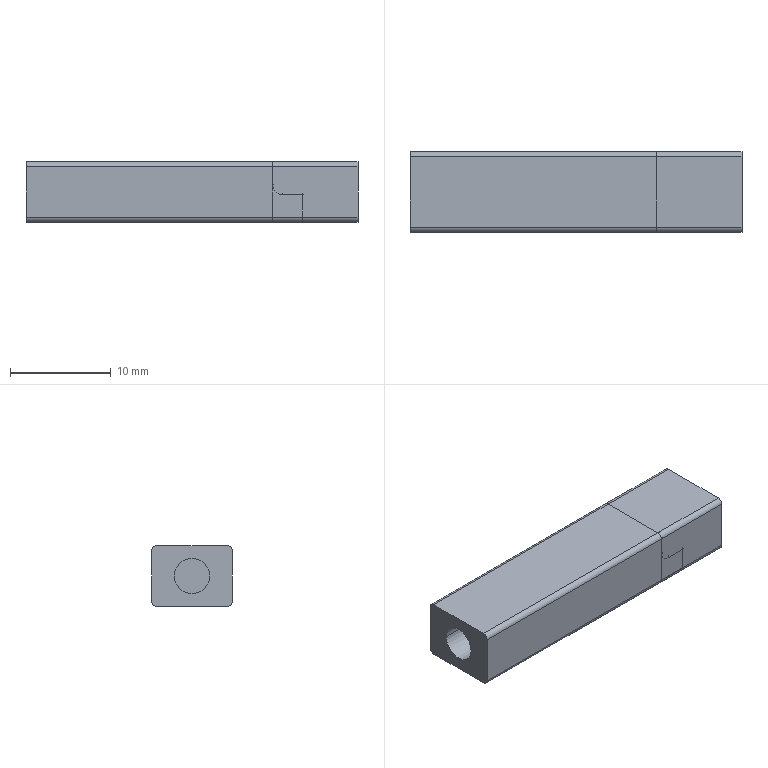NC program | NX | posted with a generic post | part box 33 x 8 x 6 mm
Whole program:
N10 G17 G21 G94 G90
(FLOOR_WALL_COPY , TOOL : D63)
N12 T01 M6
N14 G54
N16 G17 G0 G90 X51. Y0. B0. C0. S6500 M3
N18 G43 Z30. H1
N20 Z6.
N22 G94 G1 Z3. F1250.
N24 X48.
N26 X-48.
N28 X-51.
N30 Z6.
N32 G0 Z30.
N34 X51.
N36 Z5.
N38 G1 Z2.
N40 X48.
N42 X-48.
N44 X-51.
N46 Z5.
N48 G0 Z30.
N50 X51.
N52 Z4.
N54 G1 Z1.
N56 X48.
N58 X-48.
N60 X-51.
N62 Z4.
N64 G0 Z30.
N66 X51.
N68 Z3.
N70 G1 Z0.
N72 X48.
N74 X-48.
N76 X-51.
N78 Z3.
N80 G0 Z30.
N82 M5
(ZLEVEL_PROFILE_COPY_1_COPY , TOOL : D6R0.5)
N84 T08 M6
N86 G54
N88 G17 G0 G90 X20.802 Y-7.176 B0. C0. S9500 M3
N90 G43 Z30. H8
N92 Z1.485
N94 G94 G1 Z-0.016 F1000.
N96 X20.325 Y-6.384
N98 G3 X19.8 Y-6.094 R0.6
N100 G1 X16.75 Y-6.15 F3000.
N102 X16.5 Y-6.175
N104 X8.
N106 X7.77
N108 X-16.5
N110 X-19.8 Y-6.117
N112 Y-6.149 Z-0.025
N114 Y-6.184 Z-0.035
N116 X-17.095 Y-6.229
N118 X-16.5 Y-6.263
N120 X7.77
N122 X8.
N124 X16.5
N126 X17.095 Y-6.216
N128 X19.8 Y-6.191
N130 X19.799 Y-6.236 Z-0.048
N132 Y-6.257 Z-0.06
N134 G3 X16.5 Y-6.341 R27.281
N136 G1 X8.
N138 X7.77
N140 X-16.5
N142 G3 X-19.8 Y-6.243 R36.28
N144 G1 Y-6.288 Z-0.076
N146 Y-6.319 Z-0.092
N148 G2 X-16.5 Y-6.419 R40.311
N150 G1 X7.77
N152 X8.
N154 X16.5
N156 G2 X19.8 Y-6.341 R28.4
N158 G1 X19.799 Y-6.384 Z-0.111
N160 Y-6.419 Z-0.131
N162 G3 X16.5 Y-6.495 R27.002
N164 G1 X-16.5
N166 G3 X-19.8 Y-6.395 R34.53
N168 G1 Y-6.441 Z-0.155
N170 Y-6.476 Z-0.178
N172 G2 X-16.5 Y-6.57 R36.555
N174 G1 X16.5
N176 G2 X19.799 Y-6.491 R29.307
N178 G1 Y-6.533 Z-0.206
N180 X19.8 Y-6.565 Z-0.234
N182 G3 X16.5 Y-6.643 R33.342
N184 G1 X8.
N186 X7.943
N188 X-16.5
N190 G3 X-19.8 Y-6.565 R39.359
N192 G1 Y-6.609 Z-0.266
N194 Y-6.649 Z-0.299
N196 G2 X-16.5 Y-6.713 R53.479
N198 G1 X7.77
N200 X8.
N202 X16.5
N204 G2 X19.8 Y-6.645 R40.889
N206 G1 Y-6.684 Z-0.335
N208 Y-6.718 Z-0.371
N210 G3 X16.5 Y-6.778 R44.496
N212 G1 X8.
N214 X7.77
N216 X-16.5
N218 G3 X-19.8 Y-6.718 R50.386
N220 G1 Y-6.748 Z-0.411
N222 Y-6.773 Z-0.45
N224 G2 X-16.5 Y-6.835 R48.85
N226 G1 X7.77
N228 X8.
N230 X16.5
N232 G2 X19.801 Y-6.774 R46.789
N234 G1 X19.802 Y-6.805 Z-0.493
N236 X19.803 Y-6.833 Z-0.535
N238 G3 X16.5 Y-6.886 R71.351
N240 G1 X8.
N242 X7.77
N244 X-16.5
N246 G3 X-19.8 Y-6.832 R61.689
N248 G1 Y-6.861 Z-0.58
N250 Y-6.877 Z-0.625
N252 G2 X-16.5 Y-6.927 R70.469
N254 G1 X5.698
N256 X8.
N258 X16.5
N260 G2 X18.496 Y-6.888 R50.042
N262 G1 X19.512
N264 X19.803 Y-6.884
N266 X19.802 Y-6.906 Z-0.672
N268 Y-6.93 Z-0.72
N270 G3 X16.5 Y-6.96 R106.868
N272 G1 X8.
N274 X5.008
N276 X-16.5
N278 G3 X-19.8 Y-6.919 R84.242
N280 G1 Y-6.935 Z-0.768
N282 Y-6.944 Z-0.817
N284 G2 X-16.5 Y-6.983 R97.092
N286 G1 X5.008
N288 X7.77 Y-6.978
N290 X8. Y-6.983
N292 X16.5
N294 X17.095 Y-6.972
N296 X19.801 Y-6.964
N298 Y-6.974 Z-0.866
N300 Y-6.989 Z-0.916
N302 X17.095 Y-6.992
N304 X16.5 Y-6.996
N306 X8.
N308 X5.008
N310 X-16.5
N312 G3 X-19.8 Y-6.963 R100.064
N314 G1 X-19.799 Y-6.969 Z-1.015
N316 G2 X-16.404 Y-6.999 R144.074
N318 G1 X19.798
N320 Z-1.115
N322 X-16.404
N324 G3 X-19.801 Y-6.97 R159.028
N326 G1 Y-6.972 Z-1.211
N328 G2 X-16.404 Y-6.999 R170.497
N330 G1 X19.798
N332 Z-1.308
N334 X-16.404
N336 G3 X-19.801 Y-6.973 R192.987
N338 G1 Z-1.404
N340 G2 X-16.404 Y-6.999 R224.29
N342 G1 X19.798
N344 Z-1.5
N346 X-16.404
N348 G3 X-19.801 Y-6.974 R250.916
N350 X-20.321 Y-7.274 R0.6
N352 G1 X-20.775 Y-8.06
N354 Z0.
N356 G0 Z30.
N358 X-20.771 Y7.196
N360 Z1.485
N362 G1 Z-0.016 F1000.
N364 X-20.32 Y6.417
N366 G3 X-19.8 Y6.118 R0.6
N368 G1 X-19.512 F3000.
N370 X-16.75 Y6.151
N372 X-16.5 Y6.175
N374 X16.5
N376 X16.75 Y6.157
N378 X19.797 Y6.113
N380 X19.799 Y6.158 Z-0.025
N382 X19.801 Y6.186 Z-0.035
N384 X17.095 Y6.225
N386 X16.5 Y6.263
N388 X-16.5
N390 X-17.095 Y6.22
N392 X-19.8 Y6.187
N394 Y6.226 Z-0.048
N396 Y6.249 Z-0.06
N398 G3 X-16.5 Y6.341 R32.302
N400 G1 X16.5
N402 G3 X19.801 Y6.247 R35.553
N404 G1 X19.8 Y6.293 Z-0.076
N406 Y6.326 Z-0.092
N408 G2 X16.5 Y6.419 R39.825
N410 G1 X-16.5
N412 G2 X-19.8 Y6.33 R37.098
N414 G1 Y6.374 Z-0.111
N416 Y6.403 Z-0.131
N418 G3 X-16.5 Y6.495 R38.186
N420 G1 X16.5
N422 G3 X19.8 Y6.4 R33.643
N424 G1 Y6.447 Z-0.155
N426 Y6.478 Z-0.178
N428 G2 X16.5 Y6.57 R35.707
N430 G1 X-16.5
N432 G2 X-19.8 Y6.481 R36.72
N434 G1 Y6.528 Z-0.206
N436 Y6.562 Z-0.234
N438 G3 X-16.5 Y6.643 R39.006
N440 G1 X16.5
N442 G3 X19.8 Y6.565 R35.114
N444 G1 Y6.609 Z-0.266
N446 Y6.649 Z-0.299
N448 G2 X16.5 Y6.713 R39.085
N450 G1 X-16.5
N452 G2 X-19.8 Y6.644 R52.754
N454 G1 Y6.684 Z-0.335
N456 Y6.718 Z-0.371
N458 G3 X-16.5 Y6.778 R51.561
N460 G1 X16.5
N462 G3 X19.8 Y6.72 R45.061
N464 G1 X19.799 Y6.751 Z-0.411
N466 Y6.779 Z-0.45
N468 G2 X16.5 Y6.835 R42.469
N470 G1 X-16.5
N472 G2 X-19.8 Y6.773 R53.037
N474 G1 Y6.805 Z-0.493
N476 Y6.832 Z-0.535
N478 G3 X-16.5 Y6.886 R74.092
N480 G1 X16.5
N482 G3 X19.797 Y6.842 R49.587
N484 G1 Y6.866 Z-0.58
N486 Y6.89 Z-0.625
N488 G2 X16.5 Y6.927 R59.637
N490 G1 X-16.5
N492 G2 X-19.8 Y6.883 R95.676
N494 G1 Y6.905 Z-0.672
N496 Y6.929 Z-0.72
N498 G3 X-16.5 Y6.96 R130.793
N500 G1 X16.5
N502 G3 X19.798 Y6.934 R84.313
N504 G1 X19.799 Y6.954 Z-0.768
N506 Y6.966 Z-0.817
N508 G2 X16.5 Y6.983 R117.26
N510 G1 X13.987
N512 X11.224 Y6.978
N514 X11. Y6.983
N516 X-16.5
N518 G2 X-19.8 Y6.964 R181.497
N520 G1 X-19.801 Y6.979 Z-0.866
N522 Y6.989 Z-0.916
N524 X-16.75 Y6.993
N526 X-16.5 Y6.996
N528 X16.5
N530 X16.75 Y6.992
N532 X19.8 Y6.989
N534 X19.799 Y6.998 Z-1.015
N536 X-19.798
N538 X-19.799 Z-1.115
N540 X19.799
N542 Z-1.211
N544 X-19.799
N546 Z-1.308
N548 X19.799
N550 Z-1.404
N552 X-19.799
N554 Z-1.5
N556 X19.799
N558 G3 X20.318 Y7.298 R0.6
N560 G1 X20.773 Y8.085
N562 Z0.
N564 G0 Z30.
N566 M5
N568 M2